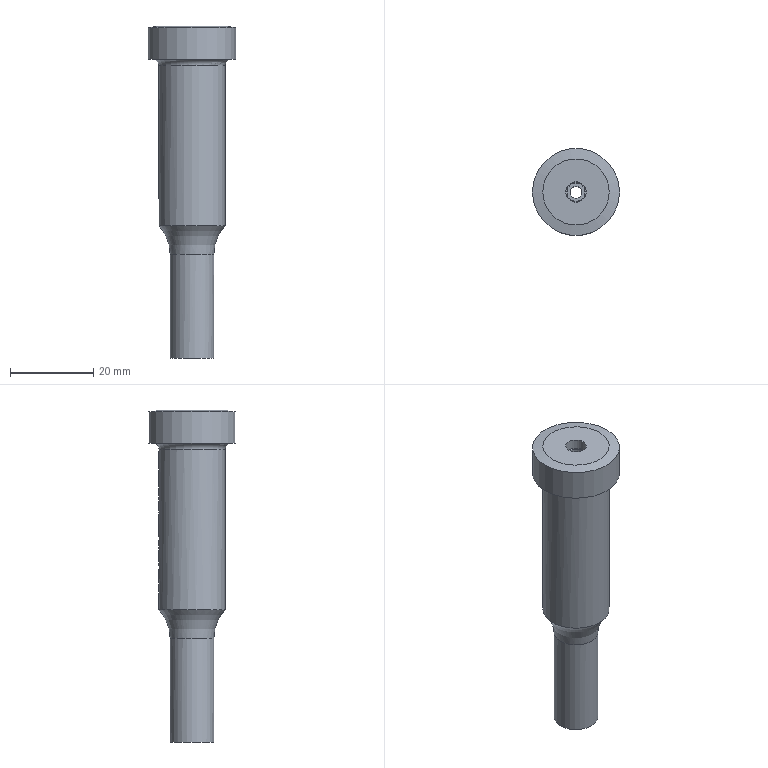Part | NX | features MI_APJAL_0250 2 | 1 solid | 212 faces | box 21 x 21 x 80 mm | volume 12964 mm3 | plane 121 | cylinder 88 | torus 2 | cone 1 | commonest cylinder face diameters 15.8 x17 16 x10 0.939 x2 1.035 x2 1.173 x2 1.229 x2